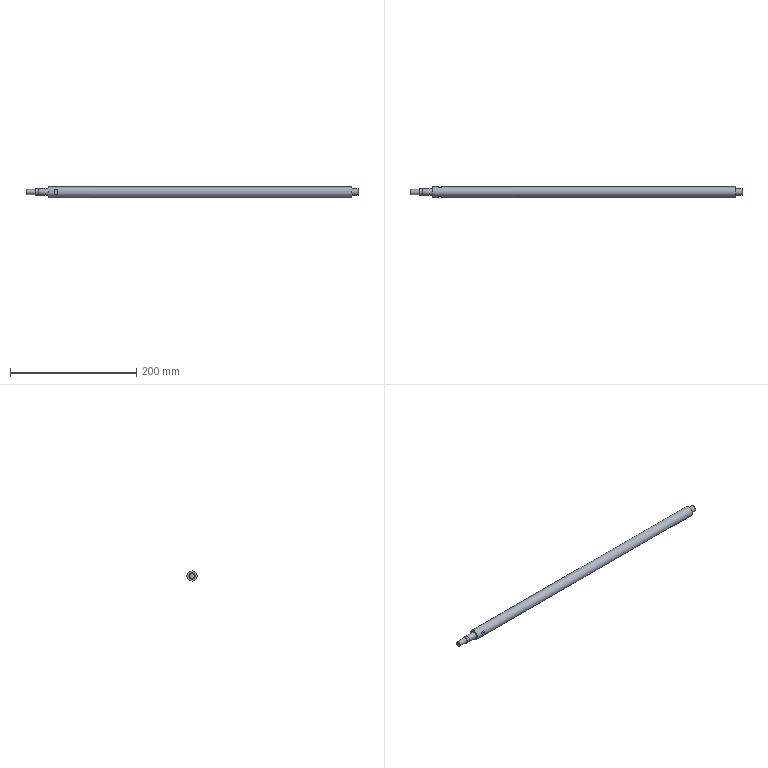Part | NX | 1 solid | 17 faces | box 525 x 16 x 16 mm | volume 99560 mm3 | plane 12 | cylinder 5 | commonest cylinder face diameters 10 x2 8 x1 9.9 x1 16 x1
STEP:
#1=CARTESIAN_POINT('',(50.,-7.,-3.873));
#2=VERTEX_POINT('',#1);
#3=CARTESIAN_POINT('',(50.,-7.,3.873));
#4=VERTEX_POINT('',#3);
#5=CARTESIAN_POINT('',(50.,0.,0.));
#6=DIRECTION('',(-1.,0.,0.));
#7=DIRECTION('',(0.,0.,-1.));
#8=AXIS2_PLACEMENT_3D('',#5,#6,#7);
#9=CIRCLE('',#8,8.);
#10=EDGE_CURVE('',#2,#4,#9,.T.);
#11=ORIENTED_EDGE('',*,*,#10,.F.);
#12=CARTESIAN_POINT('',(45.,-7.,-3.873));
#13=VERTEX_POINT('',#12);
#14=CARTESIAN_POINT('',(355.,-7.,-3.873));
#15=DIRECTION('',(1.,0.,0.));
#16=VECTOR('',#15,1.);
#17=LINE('',#14,#16);
#18=EDGE_CURVE('',#13,#2,#17,.T.);
#19=ORIENTED_EDGE('',*,*,#18,.F.);
#20=CARTESIAN_POINT('',(45.,-7.,3.873));
#21=VERTEX_POINT('',#20);
#22=CARTESIAN_POINT('',(45.,0.,0.));
#23=DIRECTION('',(1.,0.,0.));
#24=DIRECTION('',(0.,0.,1.));
#25=AXIS2_PLACEMENT_3D('',#22,#23,#24);
#26=CIRCLE('',#25,8.);
#27=EDGE_CURVE('',#21,#13,#26,.T.);
#28=ORIENTED_EDGE('',*,*,#27,.F.);
#29=CARTESIAN_POINT('',(355.,-7.,3.873));
#30=DIRECTION('',(-1.,0.,0.));
#31=VECTOR('',#30,1.);
#32=LINE('',#29,#31);
#33=EDGE_CURVE('',#4,#21,#32,.T.);
#34=ORIENTED_EDGE('',*,*,#33,.F.);
#35=EDGE_LOOP('',(#11,#19,#28,#34));
#36=FACE_BOUND('',#35,.T.);
#37=CARTESIAN_POINT('',(515.,0.,8.));
#38=VERTEX_POINT('',#37);
#39=CARTESIAN_POINT('',(515.,0.,0.));
#40=DIRECTION('',(-1.,0.,0.));
#41=DIRECTION('',(0.,0.,1.));
#42=AXIS2_PLACEMENT_3D('',#39,#40,#41);
#43=CIRCLE('',#42,8.);
#44=EDGE_CURVE('',#38,#38,#43,.T.);
#45=ORIENTED_EDGE('',*,*,#44,.T.);
#46=EDGE_LOOP('',(#45));
#47=FACE_BOUND('',#46,.T.);
#48=CARTESIAN_POINT('',(35.,0.,8.));
#49=VERTEX_POINT('',#48);
#50=CARTESIAN_POINT('',(35.,0.,0.));
#51=DIRECTION('',(-1.,0.,0.));
#52=DIRECTION('',(0.,0.,1.));
#53=AXIS2_PLACEMENT_3D('',#50,#51,#52);
#54=CIRCLE('',#53,8.);
#55=EDGE_CURVE('',#49,#49,#54,.T.);
#56=ORIENTED_EDGE('',*,*,#55,.F.);
#57=EDGE_LOOP('',(#56));
#58=FACE_BOUND('',#57,.T.);
#59=CARTESIAN_POINT('',(45.,7.,-3.873));
#60=VERTEX_POINT('',#59);
#61=CARTESIAN_POINT('',(50.,7.,-3.873));
#62=VERTEX_POINT('',#61);
#63=CARTESIAN_POINT('',(355.,7.,-3.873));
#64=DIRECTION('',(1.,0.,0.));
#65=VECTOR('',#64,1.);
#66=LINE('',#63,#65);
#67=EDGE_CURVE('',#60,#62,#66,.T.);
#68=ORIENTED_EDGE('',*,*,#67,.T.);
#69=CARTESIAN_POINT('',(50.,7.,3.873));
#70=VERTEX_POINT('',#69);
#71=CARTESIAN_POINT('',(50.,0.,0.));
#72=DIRECTION('',(1.,0.,0.));
#73=DIRECTION('',(0.,0.,1.));
#74=AXIS2_PLACEMENT_3D('',#71,#72,#73);
#75=CIRCLE('',#74,8.);
#76=EDGE_CURVE('',#62,#70,#75,.T.);
#77=ORIENTED_EDGE('',*,*,#76,.T.);
#78=CARTESIAN_POINT('',(45.,7.,3.873));
#79=VERTEX_POINT('',#78);
#80=CARTESIAN_POINT('',(355.,7.,3.873));
#81=DIRECTION('',(-1.,0.,0.));
#82=VECTOR('',#81,1.);
#83=LINE('',#80,#82);
#84=EDGE_CURVE('',#70,#79,#83,.T.);
#85=ORIENTED_EDGE('',*,*,#84,.T.);
#86=CARTESIAN_POINT('',(45.,0.,0.));
#87=DIRECTION('',(-1.,0.,0.));
#88=DIRECTION('',(0.,0.,-1.));
#89=AXIS2_PLACEMENT_3D('',#86,#87,#88);
#90=CIRCLE('',#89,8.);
#91=EDGE_CURVE('',#79,#60,#90,.T.);
#92=ORIENTED_EDGE('',*,*,#91,.T.);
#93=EDGE_LOOP('',(#68,#77,#85,#92));
#94=FACE_BOUND('',#93,.T.);
#95=CARTESIAN_POINT('',(355.,0.,0.));
#96=DIRECTION('',(-1.,0.,0.));
#97=DIRECTION('',(0.,0.,-1.));
#98=AXIS2_PLACEMENT_3D('',#95,#96,#97);
#99=CYLINDRICAL_SURFACE('',#98,8.);
#100=ADVANCED_FACE('',(#36,#47,#58,#94),#99,.T.);
#101=CARTESIAN_POINT('',(0.,0.,4.));
#102=VERTEX_POINT('',#101);
#103=CARTESIAN_POINT('',(0.,0.,0.));
#104=DIRECTION('',(-1.,0.,0.));
#105=DIRECTION('',(0.,0.,1.));
#106=AXIS2_PLACEMENT_3D('',#103,#104,#105);
#107=CIRCLE('',#106,4.);
#108=EDGE_CURVE('',#102,#102,#107,.T.);
#109=ORIENTED_EDGE('',*,*,#108,.T.);
#110=EDGE_LOOP('',(#109));
#111=FACE_OUTER_BOUND('',#110,.T.);
#112=CARTESIAN_POINT('',(0.,0.,0.));
#113=DIRECTION('',(-1.,0.,0.));
#114=DIRECTION('',(0.,0.,-1.));
#115=AXIS2_PLACEMENT_3D('',#112,#113,#114);
#116=PLANE('',#115);
#117=ADVANCED_FACE('',(#111),#116,.T.);
#118=CARTESIAN_POINT('',(15.,0.,4.));
#119=VERTEX_POINT('',#118);
#120=CARTESIAN_POINT('',(15.,0.,0.));
#121=DIRECTION('',(-1.,0.,0.));
#122=DIRECTION('',(0.,0.,1.));
#123=AXIS2_PLACEMENT_3D('',#120,#121,#122);
#124=CIRCLE('',#123,4.);
#125=EDGE_CURVE('',#119,#119,#124,.T.);
#126=ORIENTED_EDGE('',*,*,#125,.T.);
#127=EDGE_LOOP('',(#126));
#128=FACE_BOUND('',#127,.T.);
#129=ORIENTED_EDGE('',*,*,#108,.F.);
#130=EDGE_LOOP('',(#129));
#131=FACE_BOUND('',#130,.T.);
#132=CARTESIAN_POINT('',(355.,0.,0.));
#133=DIRECTION('',(-1.,0.,0.));
#134=DIRECTION('',(0.,0.,-1.));
#135=AXIS2_PLACEMENT_3D('',#132,#133,#134);
#136=CYLINDRICAL_SURFACE('',#135,4.);
#137=ADVANCED_FACE('',(#128,#131),#136,.T.);
#138=CARTESIAN_POINT('',(15.,0.,4.95));
#139=VERTEX_POINT('',#138);
#140=CARTESIAN_POINT('',(15.,0.,0.));
#141=DIRECTION('',(-1.,0.,0.));
#142=DIRECTION('',(0.,0.,1.));
#143=AXIS2_PLACEMENT_3D('',#140,#141,#142);
#144=CIRCLE('',#143,4.95);
#145=EDGE_CURVE('',#139,#139,#144,.T.);
#146=ORIENTED_EDGE('',*,*,#145,.T.);
#147=EDGE_LOOP('',(#146));
#148=FACE_BOUND('',#147,.T.);
#149=ORIENTED_EDGE('',*,*,#125,.F.);
#150=EDGE_LOOP('',(#149));
#151=FACE_BOUND('',#150,.T.);
#152=CARTESIAN_POINT('',(15.,0.,4.));
#153=DIRECTION('',(-1.,0.,0.));
#154=DIRECTION('',(0.,0.,-1.));
#155=AXIS2_PLACEMENT_3D('',#152,#153,#154);
#156=PLANE('',#155);
#157=ADVANCED_FACE('',(#148,#151),#156,.T.);
#158=CARTESIAN_POINT('',(20.,0.,4.95));
#159=VERTEX_POINT('',#158);
#160=CARTESIAN_POINT('',(20.,0.,0.));
#161=DIRECTION('',(-1.,0.,0.));
#162=DIRECTION('',(0.,0.,1.));
#163=AXIS2_PLACEMENT_3D('',#160,#161,#162);
#164=CIRCLE('',#163,4.95);
#165=EDGE_CURVE('',#159,#159,#164,.T.);
#166=ORIENTED_EDGE('',*,*,#165,.T.);
#167=EDGE_LOOP('',(#166));
#168=FACE_BOUND('',#167,.T.);
#169=ORIENTED_EDGE('',*,*,#145,.F.);
#170=EDGE_LOOP('',(#169));
#171=FACE_BOUND('',#170,.T.);
#172=CARTESIAN_POINT('',(355.,0.,0.));
#173=DIRECTION('',(-1.,0.,0.));
#174=DIRECTION('',(0.,0.,-1.));
#175=AXIS2_PLACEMENT_3D('',#172,#173,#174);
#176=CYLINDRICAL_SURFACE('',#175,4.95);
#177=ADVANCED_FACE('',(#168,#171),#176,.T.);
#178=CARTESIAN_POINT('',(20.,0.,5.));
#179=VERTEX_POINT('',#178);
#180=CARTESIAN_POINT('',(20.,0.,0.));
#181=DIRECTION('',(-1.,0.,0.));
#182=DIRECTION('',(0.,0.,1.));
#183=AXIS2_PLACEMENT_3D('',#180,#181,#182);
#184=CIRCLE('',#183,5.);
#185=EDGE_CURVE('',#179,#179,#184,.T.);
#186=ORIENTED_EDGE('',*,*,#185,.T.);
#187=EDGE_LOOP('',(#186));
#188=FACE_BOUND('',#187,.T.);
#189=ORIENTED_EDGE('',*,*,#165,.F.);
#190=EDGE_LOOP('',(#189));
#191=FACE_BOUND('',#190,.T.);
#192=CARTESIAN_POINT('',(20.,0.,4.95));
#193=DIRECTION('',(-1.,0.,0.));
#194=DIRECTION('',(0.,0.,-1.));
#195=AXIS2_PLACEMENT_3D('',#192,#193,#194);
#196=PLANE('',#195);
#197=ADVANCED_FACE('',(#188,#191),#196,.T.);
#198=CARTESIAN_POINT('',(35.,0.,5.));
#199=VERTEX_POINT('',#198);
#200=CARTESIAN_POINT('',(35.,0.,0.));
#201=DIRECTION('',(-1.,0.,0.));
#202=DIRECTION('',(0.,0.,1.));
#203=AXIS2_PLACEMENT_3D('',#200,#201,#202);
#204=CIRCLE('',#203,5.);
#205=EDGE_CURVE('',#199,#199,#204,.T.);
#206=ORIENTED_EDGE('',*,*,#205,.T.);
#207=EDGE_LOOP('',(#206));
#208=FACE_BOUND('',#207,.T.);
#209=ORIENTED_EDGE('',*,*,#185,.F.);
#210=EDGE_LOOP('',(#209));
#211=FACE_BOUND('',#210,.T.);
#212=CARTESIAN_POINT('',(355.,0.,0.));
#213=DIRECTION('',(-1.,0.,0.));
#214=DIRECTION('',(0.,0.,-1.));
#215=AXIS2_PLACEMENT_3D('',#212,#213,#214);
#216=CYLINDRICAL_SURFACE('',#215,5.);
#217=ADVANCED_FACE('',(#208,#211),#216,.T.);
#218=ORIENTED_EDGE('',*,*,#55,.T.);
#219=EDGE_LOOP('',(#218));
#220=FACE_BOUND('',#219,.T.);
#221=ORIENTED_EDGE('',*,*,#205,.F.);
#222=EDGE_LOOP('',(#221));
#223=FACE_BOUND('',#222,.T.);
#224=CARTESIAN_POINT('',(35.,0.,5.));
#225=DIRECTION('',(-1.,0.,0.));
#226=DIRECTION('',(0.,0.,-1.));
#227=AXIS2_PLACEMENT_3D('',#224,#225,#226);
#228=PLANE('',#227);
#229=ADVANCED_FACE('',(#220,#223),#228,.T.);
#230=CARTESIAN_POINT('',(515.,0.,5.));
#231=VERTEX_POINT('',#230);
#232=CARTESIAN_POINT('',(515.,0.,0.));
#233=DIRECTION('',(-1.,0.,0.));
#234=DIRECTION('',(0.,0.,1.));
#235=AXIS2_PLACEMENT_3D('',#232,#233,#234);
#236=CIRCLE('',#235,5.);
#237=EDGE_CURVE('',#231,#231,#236,.T.);
#238=ORIENTED_EDGE('',*,*,#237,.T.);
#239=EDGE_LOOP('',(#238));
#240=FACE_BOUND('',#239,.T.);
#241=ORIENTED_EDGE('',*,*,#44,.F.);
#242=EDGE_LOOP('',(#241));
#243=FACE_BOUND('',#242,.T.);
#244=CARTESIAN_POINT('',(515.,0.,8.));
#245=DIRECTION('',(1.,0.,0.));
#246=DIRECTION('',(0.,0.,1.));
#247=AXIS2_PLACEMENT_3D('',#244,#245,#246);
#248=PLANE('',#247);
#249=ADVANCED_FACE('',(#240,#243),#248,.T.);
#250=CARTESIAN_POINT('',(525.,0.,5.));
#251=VERTEX_POINT('',#250);
#252=CARTESIAN_POINT('',(525.,0.,0.));
#253=DIRECTION('',(-1.,0.,0.));
#254=DIRECTION('',(0.,0.,1.));
#255=AXIS2_PLACEMENT_3D('',#252,#253,#254);
#256=CIRCLE('',#255,5.);
#257=EDGE_CURVE('',#251,#251,#256,.T.);
#258=ORIENTED_EDGE('',*,*,#257,.T.);
#259=EDGE_LOOP('',(#258));
#260=FACE_BOUND('',#259,.T.);
#261=ORIENTED_EDGE('',*,*,#237,.F.);
#262=EDGE_LOOP('',(#261));
#263=FACE_BOUND('',#262,.T.);
#264=CARTESIAN_POINT('',(525.,0.,0.));
#265=DIRECTION('',(-1.,0.,0.));
#266=DIRECTION('',(0.,0.,-1.));
#267=AXIS2_PLACEMENT_3D('',#264,#265,#266);
#268=CYLINDRICAL_SURFACE('',#267,5.);
#269=ADVANCED_FACE('',(#260,#263),#268,.T.);
#270=ORIENTED_EDGE('',*,*,#257,.F.);
#271=EDGE_LOOP('',(#270));
#272=FACE_OUTER_BOUND('',#271,.T.);
#273=CARTESIAN_POINT('',(525.,0.,5.));
#274=DIRECTION('',(1.,0.,0.));
#275=DIRECTION('',(0.,0.,1.));
#276=AXIS2_PLACEMENT_3D('',#273,#274,#275);
#277=PLANE('',#276);
#278=ADVANCED_FACE('',(#272),#277,.T.);
#279=CARTESIAN_POINT('',(45.,7.,20.));
#280=DIRECTION('',(0.,0.,1.));
#281=VECTOR('',#280,1.);
#282=LINE('',#279,#281);
#283=EDGE_CURVE('',#60,#79,#282,.T.);
#284=ORIENTED_EDGE('',*,*,#283,.F.);
#285=ORIENTED_EDGE('',*,*,#91,.F.);
#286=EDGE_LOOP('',(#284,#285));
#287=FACE_OUTER_BOUND('',#286,.T.);
#288=CARTESIAN_POINT('',(45.,8.,20.));
#289=DIRECTION('',(1.,0.,0.));
#290=DIRECTION('',(0.,0.,1.));
#291=AXIS2_PLACEMENT_3D('',#288,#289,#290);
#292=PLANE('',#291);
#293=ADVANCED_FACE('',(#287),#292,.T.);
#294=ORIENTED_EDGE('',*,*,#283,.T.);
#295=ORIENTED_EDGE('',*,*,#84,.F.);
#296=CARTESIAN_POINT('',(50.,7.,20.));
#297=DIRECTION('',(0.,0.,1.));
#298=VECTOR('',#297,1.);
#299=LINE('',#296,#298);
#300=EDGE_CURVE('',#62,#70,#299,.T.);
#301=ORIENTED_EDGE('',*,*,#300,.F.);
#302=ORIENTED_EDGE('',*,*,#67,.F.);
#303=EDGE_LOOP('',(#294,#295,#301,#302));
#304=FACE_OUTER_BOUND('',#303,.T.);
#305=CARTESIAN_POINT('',(45.,7.,20.));
#306=DIRECTION('',(0.,1.,0.));
#307=DIRECTION('',(0.,0.,-1.));
#308=AXIS2_PLACEMENT_3D('',#305,#306,#307);
#309=PLANE('',#308);
#310=ADVANCED_FACE('',(#304),#309,.T.);
#311=ORIENTED_EDGE('',*,*,#300,.T.);
#312=ORIENTED_EDGE('',*,*,#76,.F.);
#313=EDGE_LOOP('',(#311,#312));
#314=FACE_OUTER_BOUND('',#313,.T.);
#315=CARTESIAN_POINT('',(50.,7.,20.));
#316=DIRECTION('',(-1.,0.,0.));
#317=DIRECTION('',(0.,0.,-1.));
#318=AXIS2_PLACEMENT_3D('',#315,#316,#317);
#319=PLANE('',#318);
#320=ADVANCED_FACE('',(#314),#319,.T.);
#321=CARTESIAN_POINT('',(45.,-7.,20.));
#322=DIRECTION('',(0.,0.,1.));
#323=VECTOR('',#322,1.);
#324=LINE('',#321,#323);
#325=EDGE_CURVE('',#13,#21,#324,.T.);
#326=ORIENTED_EDGE('',*,*,#325,.T.);
#327=ORIENTED_EDGE('',*,*,#27,.T.);
#328=EDGE_LOOP('',(#326,#327));
#329=FACE_OUTER_BOUND('',#328,.T.);
#330=CARTESIAN_POINT('',(45.,-8.,20.));
#331=DIRECTION('',(-1.,0.,0.));
#332=DIRECTION('',(0.,0.,-1.));
#333=AXIS2_PLACEMENT_3D('',#330,#331,#332);
#334=PLANE('',#333);
#335=ADVANCED_FACE('',(#329),#334,.F.);
#336=ORIENTED_EDGE('',*,*,#18,.T.);
#337=CARTESIAN_POINT('',(50.,-7.,20.));
#338=DIRECTION('',(0.,0.,1.));
#339=VECTOR('',#338,1.);
#340=LINE('',#337,#339);
#341=EDGE_CURVE('',#2,#4,#340,.T.);
#342=ORIENTED_EDGE('',*,*,#341,.T.);
#343=ORIENTED_EDGE('',*,*,#33,.T.);
#344=ORIENTED_EDGE('',*,*,#325,.F.);
#345=EDGE_LOOP('',(#336,#342,#343,#344));
#346=FACE_OUTER_BOUND('',#345,.T.);
#347=CARTESIAN_POINT('',(45.,-7.,20.));
#348=DIRECTION('',(0.,1.,0.));
#349=DIRECTION('',(0.,0.,-1.));
#350=AXIS2_PLACEMENT_3D('',#347,#348,#349);
#351=PLANE('',#350);
#352=ADVANCED_FACE('',(#346),#351,.F.);
#353=ORIENTED_EDGE('',*,*,#341,.F.);
#354=ORIENTED_EDGE('',*,*,#10,.T.);
#355=EDGE_LOOP('',(#353,#354));
#356=FACE_OUTER_BOUND('',#355,.T.);
#357=CARTESIAN_POINT('',(50.,-7.,20.));
#358=DIRECTION('',(1.,0.,0.));
#359=DIRECTION('',(0.,0.,1.));
#360=AXIS2_PLACEMENT_3D('',#357,#358,#359);
#361=PLANE('',#360);
#362=ADVANCED_FACE('',(#356),#361,.F.);
#363=CLOSED_SHELL('',(#100,#117,#137,#157,#177,#197,#217,#229,#249,#269,#278,#293,#310,#320,#335,#352,#362));
#364=MANIFOLD_SOLID_BREP('',#363);
#365=(LENGTH_UNIT()NAMED_UNIT(*)SI_UNIT(.MILLI.,.METRE.));
#366=UNCERTAINTY_MEASURE_WITH_UNIT(LENGTH_MEASURE(0.00002),#365,'','');
#367=(NAMED_UNIT(*)PLANE_ANGLE_UNIT()SI_UNIT($,.RADIAN.));
#368=PLANE_ANGLE_MEASURE_WITH_UNIT(PLANE_ANGLE_MEASURE(0.01745),#367);
#369=DIMENSIONAL_EXPONENTS(0.,0.,0.,0.,0.,0.,0.);
#370=(CONVERSION_BASED_UNIT('DEGREE',#368)NAMED_UNIT(#369)PLANE_ANGLE_UNIT());
#371=(NAMED_UNIT(*)SI_UNIT($,.STERADIAN.)SOLID_ANGLE_UNIT());
#372=(GEOMETRIC_REPRESENTATION_CONTEXT(3)GLOBAL_UNCERTAINTY_ASSIGNED_CONTEXT((#366))GLOBAL_UNIT_ASSIGNED_CONTEXT((#365,#370,#371))REPRESENTATION_CONTEXT('',''));
#373=ADVANCED_BREP_SHAPE_REPRESENTATION('',(#364),#372);